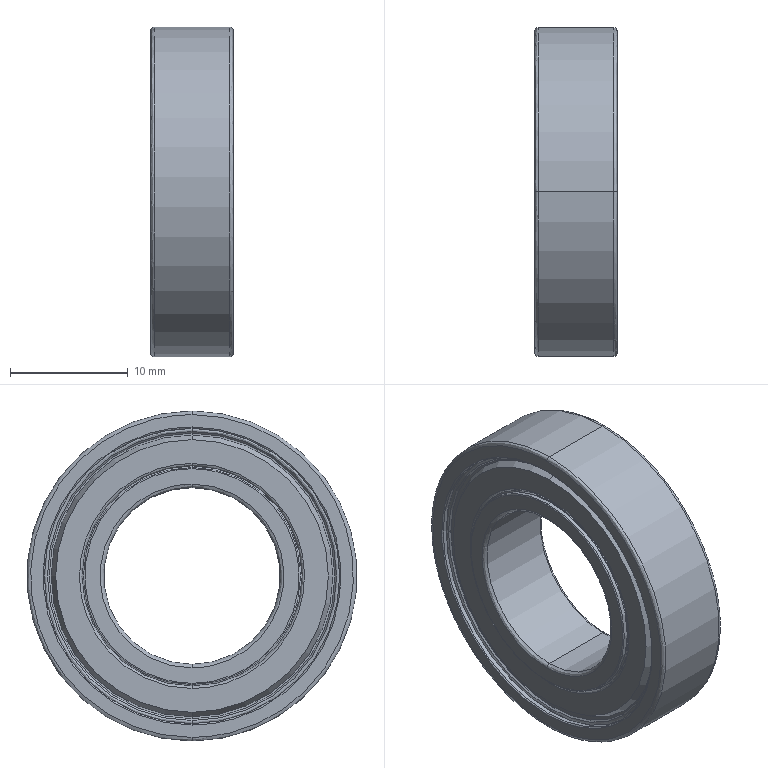Part | STEP file | BAY6902ZZ-SUS | 1 solid | 140 faces | box 7 x 28 x 28 mm | volume 2423 mm3 | spline 52 | cone 44 | cylinder 32 | plane 12 | commonest cylinder face diameters 17.8 x4 18.4 x4 18.7 x4 19.1 x4 19.3 x4 23.7 x4